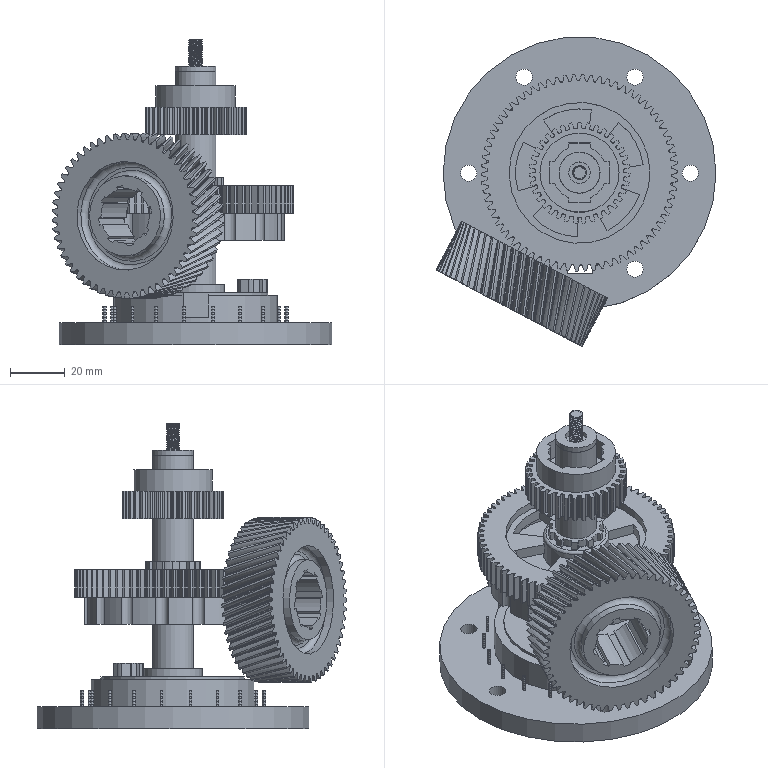Part | NX | features BREP 160, META 160, DATUM_CSYS 26, EXTRUDE 17, SKETCH 14, CYLINDER 11, FSET 3, BLEND 2, REPLACE_FACE 2, OFFSET_REGION 1, THREADS 1 | 132 solids | 1560 faces | volume 209472 mm3 | spline 802 | cylinder 378 | plane 374 | torus 6 | commonest cylinder face diameters 1 x120 67.5 x70 56.03 x55 32.5 x35 4.618 x15 65 x15